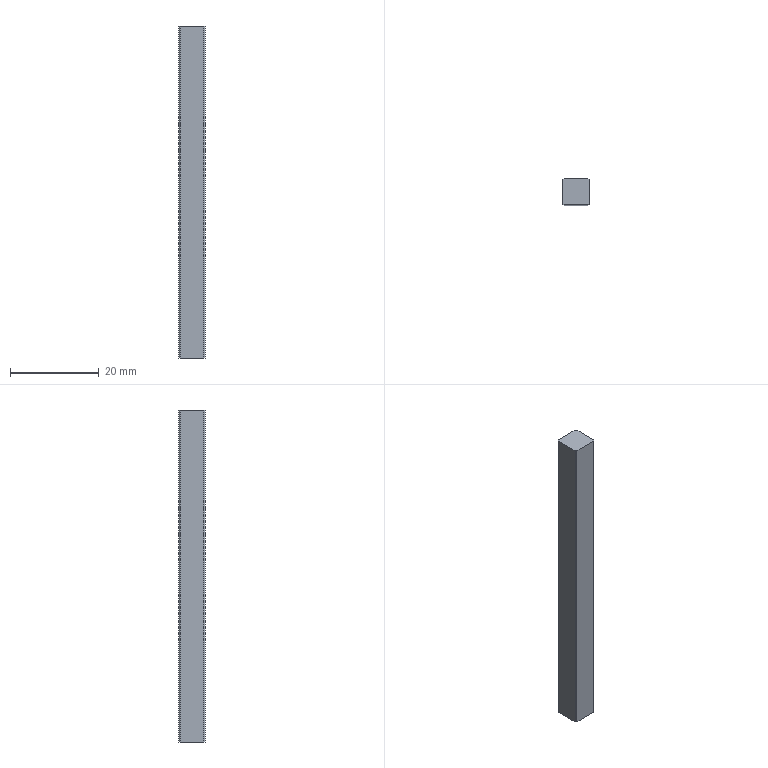Part | STEP file | Microwave Drying Flat Conveyor-Key 6x6x70 | 1 solid | 10 faces | box 6 x 6 x 75 mm | volume 2686 mm3 | plane 10
STEP:
#1=CARTESIAN_POINT('',(5.7,6.,0.));
#2=VERTEX_POINT('',#1);
#3=CARTESIAN_POINT('',(0.3,6.,0.));
#4=VERTEX_POINT('',#3);
#5=CARTESIAN_POINT('',(0.3,6.,0.));
#6=DIRECTION('',(-1.,0.,0.));
#7=VECTOR('',#6,1000.);
#8=LINE('',#5,#7);
#9=EDGE_CURVE('',#2,#4,#8,.T.);
#10=ORIENTED_EDGE('',*,*,#9,.T.);
#11=CARTESIAN_POINT('',(0.3,6.,75.));
#12=VERTEX_POINT('',#11);
#13=CARTESIAN_POINT('',(0.3,6.,75.));
#14=DIRECTION('',(0.,0.,-1.));
#15=VECTOR('',#14,1000.);
#16=LINE('',#13,#15);
#17=EDGE_CURVE('',#12,#4,#16,.T.);
#18=ORIENTED_EDGE('',*,*,#17,.F.);
#19=CARTESIAN_POINT('',(5.7,6.,75.));
#20=VERTEX_POINT('',#19);
#21=CARTESIAN_POINT('',(0.3,6.,75.));
#22=DIRECTION('',(-1.,0.,0.));
#23=VECTOR('',#22,1000.);
#24=LINE('',#21,#23);
#25=EDGE_CURVE('',#20,#12,#24,.T.);
#26=ORIENTED_EDGE('',*,*,#25,.F.);
#27=CARTESIAN_POINT('',(5.7,6.,75.));
#28=DIRECTION('',(0.,0.,-1.));
#29=VECTOR('',#28,1000.);
#30=LINE('',#27,#29);
#31=EDGE_CURVE('',#20,#2,#30,.T.);
#32=ORIENTED_EDGE('',*,*,#31,.T.);
#33=EDGE_LOOP('',(#10,#18,#26,#32));
#34=FACE_OUTER_BOUND('',#33,.T.);
#35=CARTESIAN_POINT('',(0.3,6.,75.));
#36=DIRECTION('',(0.,-1.,0.));
#37=DIRECTION('',(0.,0.,-1.));
#38=AXIS2_PLACEMENT_3D('',#35,#36,#37);
#39=PLANE('',#38);
#40=ADVANCED_FACE('',(#34),#39,.F.);
#41=CARTESIAN_POINT('',(0.,5.7,0.));
#42=VERTEX_POINT('',#41);
#43=CARTESIAN_POINT('',(0.,5.7,0.));
#44=DIRECTION('',(-0.7071,-0.7071,0.));
#45=VECTOR('',#44,1000.);
#46=LINE('',#43,#45);
#47=EDGE_CURVE('',#4,#42,#46,.T.);
#48=ORIENTED_EDGE('',*,*,#47,.T.);
#49=CARTESIAN_POINT('',(0.,5.7,75.));
#50=VERTEX_POINT('',#49);
#51=CARTESIAN_POINT('',(0.,5.7,75.));
#52=DIRECTION('',(0.,0.,-1.));
#53=VECTOR('',#52,1000.);
#54=LINE('',#51,#53);
#55=EDGE_CURVE('',#50,#42,#54,.T.);
#56=ORIENTED_EDGE('',*,*,#55,.F.);
#57=CARTESIAN_POINT('',(0.,5.7,75.));
#58=DIRECTION('',(-0.7071,-0.7071,0.));
#59=VECTOR('',#58,1000.);
#60=LINE('',#57,#59);
#61=EDGE_CURVE('',#12,#50,#60,.T.);
#62=ORIENTED_EDGE('',*,*,#61,.F.);
#63=ORIENTED_EDGE('',*,*,#17,.T.);
#64=EDGE_LOOP('',(#48,#56,#62,#63));
#65=FACE_OUTER_BOUND('',#64,.T.);
#66=CARTESIAN_POINT('',(0.,5.7,75.));
#67=DIRECTION('',(0.7071,-0.7071,0.));
#68=DIRECTION('',(0.7071,0.7071,0.));
#69=AXIS2_PLACEMENT_3D('',#66,#67,#68);
#70=PLANE('',#69);
#71=ADVANCED_FACE('',(#65),#70,.F.);
#72=CARTESIAN_POINT('',(0.,0.3,0.));
#73=VERTEX_POINT('',#72);
#74=CARTESIAN_POINT('',(0.,0.3,0.));
#75=DIRECTION('',(0.,-1.,0.));
#76=VECTOR('',#75,1000.);
#77=LINE('',#74,#76);
#78=EDGE_CURVE('',#42,#73,#77,.T.);
#79=ORIENTED_EDGE('',*,*,#78,.T.);
#80=CARTESIAN_POINT('',(0.,0.3,75.));
#81=VERTEX_POINT('',#80);
#82=CARTESIAN_POINT('',(0.,0.3,75.));
#83=DIRECTION('',(0.,0.,-1.));
#84=VECTOR('',#83,1000.);
#85=LINE('',#82,#84);
#86=EDGE_CURVE('',#81,#73,#85,.T.);
#87=ORIENTED_EDGE('',*,*,#86,.F.);
#88=CARTESIAN_POINT('',(0.,0.3,75.));
#89=DIRECTION('',(0.,-1.,0.));
#90=VECTOR('',#89,1000.);
#91=LINE('',#88,#90);
#92=EDGE_CURVE('',#50,#81,#91,.T.);
#93=ORIENTED_EDGE('',*,*,#92,.F.);
#94=ORIENTED_EDGE('',*,*,#55,.T.);
#95=EDGE_LOOP('',(#79,#87,#93,#94));
#96=FACE_OUTER_BOUND('',#95,.T.);
#97=CARTESIAN_POINT('',(0.,0.3,75.));
#98=DIRECTION('',(1.,0.,0.));
#99=DIRECTION('',(0.,0.,-1.));
#100=AXIS2_PLACEMENT_3D('',#97,#98,#99);
#101=PLANE('',#100);
#102=ADVANCED_FACE('',(#96),#101,.F.);
#103=CARTESIAN_POINT('',(0.3,0.,0.));
#104=VERTEX_POINT('',#103);
#105=CARTESIAN_POINT('',(0.,0.3,0.));
#106=DIRECTION('',(0.7071,-0.7071,0.));
#107=VECTOR('',#106,1000.);
#108=LINE('',#105,#107);
#109=EDGE_CURVE('',#73,#104,#108,.T.);
#110=ORIENTED_EDGE('',*,*,#109,.T.);
#111=CARTESIAN_POINT('',(0.3,0.,75.));
#112=VERTEX_POINT('',#111);
#113=CARTESIAN_POINT('',(0.3,0.,75.));
#114=DIRECTION('',(0.,0.,-1.));
#115=VECTOR('',#114,1000.);
#116=LINE('',#113,#115);
#117=EDGE_CURVE('',#112,#104,#116,.T.);
#118=ORIENTED_EDGE('',*,*,#117,.F.);
#119=CARTESIAN_POINT('',(0.,0.3,75.));
#120=DIRECTION('',(0.7071,-0.7071,0.));
#121=VECTOR('',#120,1000.);
#122=LINE('',#119,#121);
#123=EDGE_CURVE('',#81,#112,#122,.T.);
#124=ORIENTED_EDGE('',*,*,#123,.F.);
#125=ORIENTED_EDGE('',*,*,#86,.T.);
#126=EDGE_LOOP('',(#110,#118,#124,#125));
#127=FACE_OUTER_BOUND('',#126,.T.);
#128=CARTESIAN_POINT('',(0.,0.3,75.));
#129=DIRECTION('',(0.7071,0.7071,0.));
#130=DIRECTION('',(-0.7071,0.7071,0.));
#131=AXIS2_PLACEMENT_3D('',#128,#129,#130);
#132=PLANE('',#131);
#133=ADVANCED_FACE('',(#127),#132,.F.);
#134=CARTESIAN_POINT('',(5.7,0.,0.));
#135=VERTEX_POINT('',#134);
#136=CARTESIAN_POINT('',(0.3,0.,0.));
#137=DIRECTION('',(1.,0.,0.));
#138=VECTOR('',#137,1000.);
#139=LINE('',#136,#138);
#140=EDGE_CURVE('',#104,#135,#139,.T.);
#141=ORIENTED_EDGE('',*,*,#140,.T.);
#142=CARTESIAN_POINT('',(5.7,0.,75.));
#143=VERTEX_POINT('',#142);
#144=CARTESIAN_POINT('',(5.7,0.,75.));
#145=DIRECTION('',(0.,0.,-1.));
#146=VECTOR('',#145,1000.);
#147=LINE('',#144,#146);
#148=EDGE_CURVE('',#143,#135,#147,.T.);
#149=ORIENTED_EDGE('',*,*,#148,.F.);
#150=CARTESIAN_POINT('',(0.3,0.,75.));
#151=DIRECTION('',(1.,0.,0.));
#152=VECTOR('',#151,1000.);
#153=LINE('',#150,#152);
#154=EDGE_CURVE('',#112,#143,#153,.T.);
#155=ORIENTED_EDGE('',*,*,#154,.F.);
#156=ORIENTED_EDGE('',*,*,#117,.T.);
#157=EDGE_LOOP('',(#141,#149,#155,#156));
#158=FACE_OUTER_BOUND('',#157,.T.);
#159=CARTESIAN_POINT('',(0.3,0.,75.));
#160=DIRECTION('',(0.,1.,0.));
#161=DIRECTION('',(0.,0.,1.));
#162=AXIS2_PLACEMENT_3D('',#159,#160,#161);
#163=PLANE('',#162);
#164=ADVANCED_FACE('',(#158),#163,.F.);
#165=CARTESIAN_POINT('',(6.,0.3,0.));
#166=VERTEX_POINT('',#165);
#167=CARTESIAN_POINT('',(5.7,0.,0.));
#168=DIRECTION('',(0.7071,0.7071,0.));
#169=VECTOR('',#168,1000.);
#170=LINE('',#167,#169);
#171=EDGE_CURVE('',#135,#166,#170,.T.);
#172=ORIENTED_EDGE('',*,*,#171,.T.);
#173=CARTESIAN_POINT('',(6.,0.3,75.));
#174=VERTEX_POINT('',#173);
#175=CARTESIAN_POINT('',(6.,0.3,75.));
#176=DIRECTION('',(0.,0.,-1.));
#177=VECTOR('',#176,1000.);
#178=LINE('',#175,#177);
#179=EDGE_CURVE('',#174,#166,#178,.T.);
#180=ORIENTED_EDGE('',*,*,#179,.F.);
#181=CARTESIAN_POINT('',(5.7,0.,75.));
#182=DIRECTION('',(0.7071,0.7071,0.));
#183=VECTOR('',#182,1000.);
#184=LINE('',#181,#183);
#185=EDGE_CURVE('',#143,#174,#184,.T.);
#186=ORIENTED_EDGE('',*,*,#185,.F.);
#187=ORIENTED_EDGE('',*,*,#148,.T.);
#188=EDGE_LOOP('',(#172,#180,#186,#187));
#189=FACE_OUTER_BOUND('',#188,.T.);
#190=CARTESIAN_POINT('',(5.7,0.,75.));
#191=DIRECTION('',(-0.7071,0.7071,0.));
#192=DIRECTION('',(-0.7071,-0.7071,0.));
#193=AXIS2_PLACEMENT_3D('',#190,#191,#192);
#194=PLANE('',#193);
#195=ADVANCED_FACE('',(#189),#194,.F.);
#196=CARTESIAN_POINT('',(6.,5.7,0.));
#197=VERTEX_POINT('',#196);
#198=CARTESIAN_POINT('',(6.,0.3,0.));
#199=DIRECTION('',(0.,1.,0.));
#200=VECTOR('',#199,1000.);
#201=LINE('',#198,#200);
#202=EDGE_CURVE('',#166,#197,#201,.T.);
#203=ORIENTED_EDGE('',*,*,#202,.T.);
#204=CARTESIAN_POINT('',(6.,5.7,75.));
#205=VERTEX_POINT('',#204);
#206=CARTESIAN_POINT('',(6.,5.7,75.));
#207=DIRECTION('',(0.,0.,-1.));
#208=VECTOR('',#207,1000.);
#209=LINE('',#206,#208);
#210=EDGE_CURVE('',#205,#197,#209,.T.);
#211=ORIENTED_EDGE('',*,*,#210,.F.);
#212=CARTESIAN_POINT('',(6.,0.3,75.));
#213=DIRECTION('',(0.,1.,0.));
#214=VECTOR('',#213,1000.);
#215=LINE('',#212,#214);
#216=EDGE_CURVE('',#174,#205,#215,.T.);
#217=ORIENTED_EDGE('',*,*,#216,.F.);
#218=ORIENTED_EDGE('',*,*,#179,.T.);
#219=EDGE_LOOP('',(#203,#211,#217,#218));
#220=FACE_OUTER_BOUND('',#219,.T.);
#221=CARTESIAN_POINT('',(6.,0.3,75.));
#222=DIRECTION('',(-1.,0.,0.));
#223=DIRECTION('',(0.,0.,1.));
#224=AXIS2_PLACEMENT_3D('',#221,#222,#223);
#225=PLANE('',#224);
#226=ADVANCED_FACE('',(#220),#225,.F.);
#227=CARTESIAN_POINT('',(5.7,6.,0.));
#228=DIRECTION('',(-0.7071,0.7071,0.));
#229=VECTOR('',#228,1000.);
#230=LINE('',#227,#229);
#231=EDGE_CURVE('',#197,#2,#230,.T.);
#232=ORIENTED_EDGE('',*,*,#231,.T.);
#233=ORIENTED_EDGE('',*,*,#31,.F.);
#234=CARTESIAN_POINT('',(5.7,6.,75.));
#235=DIRECTION('',(-0.7071,0.7071,0.));
#236=VECTOR('',#235,1000.);
#237=LINE('',#234,#236);
#238=EDGE_CURVE('',#205,#20,#237,.T.);
#239=ORIENTED_EDGE('',*,*,#238,.F.);
#240=ORIENTED_EDGE('',*,*,#210,.T.);
#241=EDGE_LOOP('',(#232,#233,#239,#240));
#242=FACE_OUTER_BOUND('',#241,.T.);
#243=CARTESIAN_POINT('',(5.7,6.,75.));
#244=DIRECTION('',(-0.7071,-0.7071,0.));
#245=DIRECTION('',(0.7071,-0.7071,0.));
#246=AXIS2_PLACEMENT_3D('',#243,#244,#245);
#247=PLANE('',#246);
#248=ADVANCED_FACE('',(#242),#247,.F.);
#249=ORIENTED_EDGE('',*,*,#25,.T.);
#250=ORIENTED_EDGE('',*,*,#61,.T.);
#251=ORIENTED_EDGE('',*,*,#92,.T.);
#252=ORIENTED_EDGE('',*,*,#123,.T.);
#253=ORIENTED_EDGE('',*,*,#154,.T.);
#254=ORIENTED_EDGE('',*,*,#185,.T.);
#255=ORIENTED_EDGE('',*,*,#216,.T.);
#256=ORIENTED_EDGE('',*,*,#238,.T.);
#257=EDGE_LOOP('',(#249,#250,#251,#252,#253,#254,#255,#256));
#258=FACE_OUTER_BOUND('',#257,.T.);
#259=CARTESIAN_POINT('',(0.,0.,75.));
#260=DIRECTION('',(0.,0.,1.));
#261=DIRECTION('',(1.,0.,0.));
#262=AXIS2_PLACEMENT_3D('',#259,#260,#261);
#263=PLANE('',#262);
#264=ADVANCED_FACE('',(#258),#263,.T.);
#265=ORIENTED_EDGE('',*,*,#9,.F.);
#266=ORIENTED_EDGE('',*,*,#231,.F.);
#267=ORIENTED_EDGE('',*,*,#202,.F.);
#268=ORIENTED_EDGE('',*,*,#171,.F.);
#269=ORIENTED_EDGE('',*,*,#140,.F.);
#270=ORIENTED_EDGE('',*,*,#109,.F.);
#271=ORIENTED_EDGE('',*,*,#78,.F.);
#272=ORIENTED_EDGE('',*,*,#47,.F.);
#273=EDGE_LOOP('',(#265,#266,#267,#268,#269,#270,#271,#272));
#274=FACE_OUTER_BOUND('',#273,.T.);
#275=CARTESIAN_POINT('',(0.,0.,0.));
#276=DIRECTION('',(0.,0.,1.));
#277=DIRECTION('',(1.,0.,0.));
#278=AXIS2_PLACEMENT_3D('',#275,#276,#277);
#279=PLANE('',#278);
#280=ADVANCED_FACE('',(#274),#279,.F.);
#281=CLOSED_SHELL('',(#40,#71,#102,#133,#164,#195,#226,#248,#264,#280));
#282=MANIFOLD_SOLID_BREP('',#281);
#283=CARTESIAN_POINT('',(0.,0.,0.));
#284=DIRECTION('',(0.,0.,1.));
#285=DIRECTION('',(1.,0.,0.));
#286=AXIS2_PLACEMENT_3D('',#283,#284,#285);
#287=(LENGTH_UNIT()NAMED_UNIT(*)SI_UNIT(.MILLI.,.METRE.));
#288=UNCERTAINTY_MEASURE_WITH_UNIT(LENGTH_MEASURE(0.00001),#287,'','');
#289=(NAMED_UNIT(*)PLANE_ANGLE_UNIT()SI_UNIT($,.RADIAN.));
#290=(NAMED_UNIT(*)SI_UNIT($,.STERADIAN.)SOLID_ANGLE_UNIT());
#291=(GEOMETRIC_REPRESENTATION_CONTEXT(3)GLOBAL_UNCERTAINTY_ASSIGNED_CONTEXT((#288))GLOBAL_UNIT_ASSIGNED_CONTEXT((#287,#289,#290))REPRESENTATION_CONTEXT('',''));
#292=ADVANCED_BREP_SHAPE_REPRESENTATION('',(#282,#286),#291);